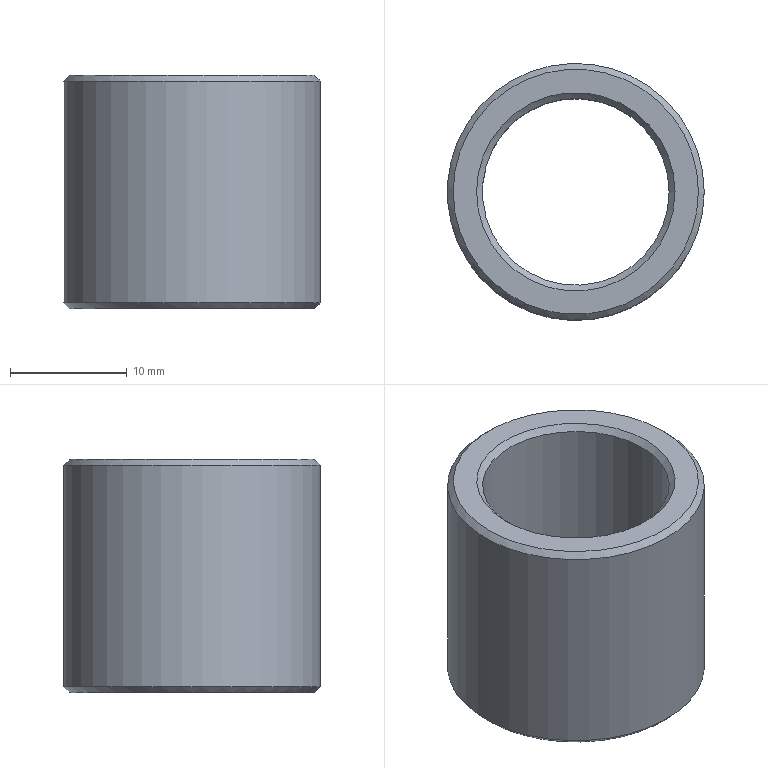Part | NX | features DATUM_CSYS 2, CHAMFER 1, DATUM_PLANE 1, EXTRUDE 1, SKETCH 1 | 1 solid | 8 faces | box 22 x 22 x 20 mm | volume 3552 mm3 | cone 4 | cylinder 2 | plane 2 | commonest cylinder face diameters 16 x1 22 x1
STEP:
#1=CARTESIAN_POINT('',(11.,0.,-9.5));
#2=VERTEX_POINT('',#1);
#3=CARTESIAN_POINT('',(0.,0.,-9.5));
#4=DIRECTION('',(0.,0.,1.));
#5=DIRECTION('',(1.,0.,0.));
#6=AXIS2_PLACEMENT_3D('',#3,#4,#5);
#7=CIRCLE('',#6,11.);
#8=EDGE_CURVE('',#2,#2,#7,.T.);
#9=ORIENTED_EDGE('',*,*,#8,.T.);
#10=EDGE_LOOP('',(#9));
#11=FACE_BOUND('',#10,.T.);
#12=CARTESIAN_POINT('',(11.,0.,9.5));
#13=VERTEX_POINT('',#12);
#14=CARTESIAN_POINT('',(0.,0.,9.5));
#15=DIRECTION('',(0.,0.,1.));
#16=DIRECTION('',(1.,0.,0.));
#17=AXIS2_PLACEMENT_3D('',#14,#15,#16);
#18=CIRCLE('',#17,11.);
#19=EDGE_CURVE('',#13,#13,#18,.F.);
#20=ORIENTED_EDGE('',*,*,#19,.T.);
#21=EDGE_LOOP('',(#20));
#22=FACE_BOUND('',#21,.T.);
#23=CARTESIAN_POINT('',(0.,0.,10.));
#24=DIRECTION('',(0.,0.,-1.));
#25=DIRECTION('',(-1.,0.,0.));
#26=AXIS2_PLACEMENT_3D('',#23,#24,#25);
#27=CYLINDRICAL_SURFACE('',#26,11.);
#28=ADVANCED_FACE('',(#11,#22),#27,.T.);
#29=CARTESIAN_POINT('',(8.,0.,-9.5));
#30=VERTEX_POINT('',#29);
#31=CARTESIAN_POINT('',(0.,0.,-9.5));
#32=DIRECTION('',(0.,0.,1.));
#33=DIRECTION('',(1.,0.,0.));
#34=AXIS2_PLACEMENT_3D('',#31,#32,#33);
#35=CIRCLE('',#34,8.);
#36=EDGE_CURVE('',#30,#30,#35,.F.);
#37=ORIENTED_EDGE('',*,*,#36,.T.);
#38=EDGE_LOOP('',(#37));
#39=FACE_BOUND('',#38,.T.);
#40=CARTESIAN_POINT('',(8.,0.,9.5));
#41=VERTEX_POINT('',#40);
#42=CARTESIAN_POINT('',(0.,0.,9.5));
#43=DIRECTION('',(0.,0.,1.));
#44=DIRECTION('',(1.,0.,0.));
#45=AXIS2_PLACEMENT_3D('',#42,#43,#44);
#46=CIRCLE('',#45,8.);
#47=EDGE_CURVE('',#41,#41,#46,.T.);
#48=ORIENTED_EDGE('',*,*,#47,.T.);
#49=EDGE_LOOP('',(#48));
#50=FACE_BOUND('',#49,.T.);
#51=CARTESIAN_POINT('',(0.,0.,10.));
#52=DIRECTION('',(0.,0.,-1.));
#53=DIRECTION('',(-1.,0.,0.));
#54=AXIS2_PLACEMENT_3D('',#51,#52,#53);
#55=CYLINDRICAL_SURFACE('',#54,8.);
#56=ADVANCED_FACE('',(#39,#50),#55,.F.);
#57=CARTESIAN_POINT('',(10.5,0.,10.));
#58=VERTEX_POINT('',#57);
#59=CARTESIAN_POINT('',(0.,0.,10.));
#60=DIRECTION('',(0.,0.,1.));
#61=DIRECTION('',(1.,0.,0.));
#62=AXIS2_PLACEMENT_3D('',#59,#60,#61);
#63=CIRCLE('',#62,10.5);
#64=EDGE_CURVE('',#58,#58,#63,.T.);
#65=ORIENTED_EDGE('',*,*,#64,.T.);
#66=EDGE_LOOP('',(#65));
#67=FACE_BOUND('',#66,.T.);
#68=CARTESIAN_POINT('',(8.5,0.,10.));
#69=VERTEX_POINT('',#68);
#70=CARTESIAN_POINT('',(0.,0.,10.));
#71=DIRECTION('',(0.,0.,1.));
#72=DIRECTION('',(1.,0.,0.));
#73=AXIS2_PLACEMENT_3D('',#70,#71,#72);
#74=CIRCLE('',#73,8.5);
#75=EDGE_CURVE('',#69,#69,#74,.F.);
#76=ORIENTED_EDGE('',*,*,#75,.T.);
#77=EDGE_LOOP('',(#76));
#78=FACE_BOUND('',#77,.T.);
#79=CARTESIAN_POINT('',(0.,0.,10.));
#80=DIRECTION('',(0.,0.,1.));
#81=DIRECTION('',(1.,0.,0.));
#82=AXIS2_PLACEMENT_3D('',#79,#80,#81);
#83=PLANE('',#82);
#84=ADVANCED_FACE('',(#67,#78),#83,.T.);
#85=CARTESIAN_POINT('',(8.5,0.,-10.));
#86=VERTEX_POINT('',#85);
#87=CARTESIAN_POINT('',(0.,0.,-10.));
#88=DIRECTION('',(0.,0.,1.));
#89=DIRECTION('',(1.,0.,0.));
#90=AXIS2_PLACEMENT_3D('',#87,#88,#89);
#91=CIRCLE('',#90,8.5);
#92=EDGE_CURVE('',#86,#86,#91,.T.);
#93=ORIENTED_EDGE('',*,*,#92,.T.);
#94=EDGE_LOOP('',(#93));
#95=FACE_BOUND('',#94,.T.);
#96=CARTESIAN_POINT('',(10.5,0.,-10.));
#97=VERTEX_POINT('',#96);
#98=CARTESIAN_POINT('',(0.,0.,-10.));
#99=DIRECTION('',(0.,0.,1.));
#100=DIRECTION('',(1.,0.,0.));
#101=AXIS2_PLACEMENT_3D('',#98,#99,#100);
#102=CIRCLE('',#101,10.5);
#103=EDGE_CURVE('',#97,#97,#102,.F.);
#104=ORIENTED_EDGE('',*,*,#103,.T.);
#105=EDGE_LOOP('',(#104));
#106=FACE_BOUND('',#105,.T.);
#107=CARTESIAN_POINT('',(0.,0.,-10.));
#108=DIRECTION('',(0.,0.,1.));
#109=DIRECTION('',(1.,0.,0.));
#110=AXIS2_PLACEMENT_3D('',#107,#108,#109);
#111=PLANE('',#110);
#112=ADVANCED_FACE('',(#95,#106),#111,.F.);
#113=ORIENTED_EDGE('',*,*,#36,.F.);
#114=EDGE_LOOP('',(#113));
#115=FACE_BOUND('',#114,.T.);
#116=ORIENTED_EDGE('',*,*,#92,.F.);
#117=EDGE_LOOP('',(#116));
#118=FACE_BOUND('',#117,.T.);
#119=CARTESIAN_POINT('',(0.,0.,-10.));
#120=DIRECTION('',(0.,0.,-1.));
#121=DIRECTION('',(-1.,0.,0.));
#122=AXIS2_PLACEMENT_3D('',#119,#120,#121);
#123=CONICAL_SURFACE('',#122,8.5,0.7854);
#124=ADVANCED_FACE('',(#115,#118),#123,.F.);
#125=ORIENTED_EDGE('',*,*,#103,.F.);
#126=EDGE_LOOP('',(#125));
#127=FACE_BOUND('',#126,.T.);
#128=ORIENTED_EDGE('',*,*,#8,.F.);
#129=EDGE_LOOP('',(#128));
#130=FACE_BOUND('',#129,.T.);
#131=CARTESIAN_POINT('',(0.,0.,-9.5));
#132=DIRECTION('',(0.,0.,1.));
#133=DIRECTION('',(1.,0.,0.));
#134=AXIS2_PLACEMENT_3D('',#131,#132,#133);
#135=CONICAL_SURFACE('',#134,11.,0.7854);
#136=ADVANCED_FACE('',(#127,#130),#135,.T.);
#137=ORIENTED_EDGE('',*,*,#19,.F.);
#138=EDGE_LOOP('',(#137));
#139=FACE_BOUND('',#138,.T.);
#140=ORIENTED_EDGE('',*,*,#64,.F.);
#141=EDGE_LOOP('',(#140));
#142=FACE_BOUND('',#141,.T.);
#143=CARTESIAN_POINT('',(0.,0.,10.));
#144=DIRECTION('',(0.,0.,-1.));
#145=DIRECTION('',(-1.,0.,0.));
#146=AXIS2_PLACEMENT_3D('',#143,#144,#145);
#147=CONICAL_SURFACE('',#146,10.5,0.7854);
#148=ADVANCED_FACE('',(#139,#142),#147,.T.);
#149=ORIENTED_EDGE('',*,*,#75,.F.);
#150=EDGE_LOOP('',(#149));
#151=FACE_BOUND('',#150,.T.);
#152=ORIENTED_EDGE('',*,*,#47,.F.);
#153=EDGE_LOOP('',(#152));
#154=FACE_BOUND('',#153,.T.);
#155=CARTESIAN_POINT('',(0.,0.,9.5));
#156=DIRECTION('',(0.,0.,1.));
#157=DIRECTION('',(1.,0.,0.));
#158=AXIS2_PLACEMENT_3D('',#155,#156,#157);
#159=CONICAL_SURFACE('',#158,8.,0.7854);
#160=ADVANCED_FACE('',(#151,#154),#159,.F.);
#161=CLOSED_SHELL('',(#28,#56,#84,#112,#124,#136,#148,#160));
#162=MANIFOLD_SOLID_BREP('',#161);
#163=(LENGTH_UNIT()NAMED_UNIT(*)SI_UNIT(.MILLI.,.METRE.));
#164=UNCERTAINTY_MEASURE_WITH_UNIT(LENGTH_MEASURE(0.00001),#163,'','');
#165=(NAMED_UNIT(*)PLANE_ANGLE_UNIT()SI_UNIT($,.RADIAN.));
#166=(NAMED_UNIT(*)SI_UNIT($,.STERADIAN.)SOLID_ANGLE_UNIT());
#167=(GEOMETRIC_REPRESENTATION_CONTEXT(3)GLOBAL_UNCERTAINTY_ASSIGNED_CONTEXT((#164))GLOBAL_UNIT_ASSIGNED_CONTEXT((#163,#165,#166))REPRESENTATION_CONTEXT('',''));
#168=ADVANCED_BREP_SHAPE_REPRESENTATION('',(#162),#167);